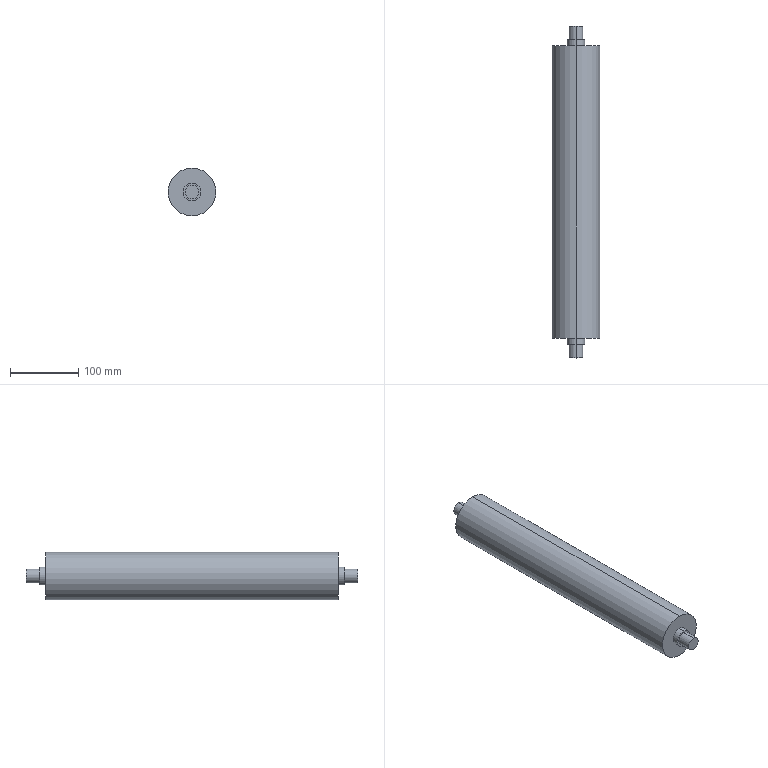Part | STEP file | 1.6米滚轮1 | 1 solid | 16 faces | box 70 x 486 x 70 mm | volume 1669260 mm3 | cylinder 10 | plane 6 | commonest cylinder face diameters 20 x4 26 x4 70 x2
STEP:
#1=CARTESIAN_POINT('',(0.,-29.,10.));
#2=VERTEX_POINT('',#1);
#3=CARTESIAN_POINT('',(0.,-29.,-10.));
#4=VERTEX_POINT('',#3);
#5=CARTESIAN_POINT('',(0.,-29.,0.));
#6=DIRECTION('',(0.,1.,0.));
#7=DIRECTION('',(0.,0.,1.));
#8=AXIS2_PLACEMENT_3D('',#5,#6,#7);
#9=CIRCLE('',#8,10.);
#10=EDGE_CURVE('',#2,#4,#9,.T.);
#11=ORIENTED_EDGE('',*,*,#10,.T.);
#12=CARTESIAN_POINT('',(0.,-9.,-10.));
#13=VERTEX_POINT('',#12);
#14=CARTESIAN_POINT('',(0.,-29.,-10.));
#15=DIRECTION('',(0.,1.,0.));
#16=VECTOR('',#15,1000.);
#17=LINE('',#14,#16);
#18=EDGE_CURVE('',#4,#13,#17,.T.);
#19=ORIENTED_EDGE('',*,*,#18,.T.);
#20=CARTESIAN_POINT('',(0.,-9.,10.));
#21=VERTEX_POINT('',#20);
#22=CARTESIAN_POINT('',(0.,-9.,0.));
#23=DIRECTION('',(0.,-1.,0.));
#24=DIRECTION('',(0.,0.,-1.));
#25=AXIS2_PLACEMENT_3D('',#22,#23,#24);
#26=CIRCLE('',#25,10.);
#27=EDGE_CURVE('',#13,#21,#26,.T.);
#28=ORIENTED_EDGE('',*,*,#27,.T.);
#29=CARTESIAN_POINT('',(0.,-29.,10.));
#30=DIRECTION('',(0.,1.,0.));
#31=VECTOR('',#30,1000.);
#32=LINE('',#29,#31);
#33=EDGE_CURVE('',#2,#21,#32,.T.);
#34=ORIENTED_EDGE('',*,*,#33,.F.);
#35=EDGE_LOOP('',(#11,#19,#28,#34));
#36=FACE_OUTER_BOUND('',#35,.T.);
#37=CARTESIAN_POINT('',(0.,-29.,0.));
#38=DIRECTION('',(0.,1.,0.));
#39=DIRECTION('',(0.,0.,1.));
#40=AXIS2_PLACEMENT_3D('',#37,#38,#39);
#41=CYLINDRICAL_SURFACE('',#40,10.);
#42=ADVANCED_FACE('',(#36),#41,.T.);
#43=CARTESIAN_POINT('',(0.,-9.,13.));
#44=VERTEX_POINT('',#43);
#45=CARTESIAN_POINT('',(0.,-9.,-13.));
#46=VERTEX_POINT('',#45);
#47=CARTESIAN_POINT('',(0.,-9.,0.));
#48=DIRECTION('',(0.,1.,0.));
#49=DIRECTION('',(0.,0.,1.));
#50=AXIS2_PLACEMENT_3D('',#47,#48,#49);
#51=CIRCLE('',#50,13.);
#52=EDGE_CURVE('',#44,#46,#51,.T.);
#53=ORIENTED_EDGE('',*,*,#52,.T.);
#54=CARTESIAN_POINT('',(0.,0.,-13.));
#55=VERTEX_POINT('',#54);
#56=CARTESIAN_POINT('',(0.,-9.,-13.));
#57=DIRECTION('',(0.,1.,0.));
#58=VECTOR('',#57,1000.);
#59=LINE('',#56,#58);
#60=EDGE_CURVE('',#46,#55,#59,.T.);
#61=ORIENTED_EDGE('',*,*,#60,.T.);
#62=CARTESIAN_POINT('',(0.,0.,13.));
#63=VERTEX_POINT('',#62);
#64=CARTESIAN_POINT('',(0.,0.,0.));
#65=DIRECTION('',(0.,1.,0.));
#66=DIRECTION('',(0.,0.,1.));
#67=AXIS2_PLACEMENT_3D('',#64,#65,#66);
#68=CIRCLE('',#67,13.);
#69=EDGE_CURVE('',#63,#55,#68,.T.);
#70=ORIENTED_EDGE('',*,*,#69,.F.);
#71=CARTESIAN_POINT('',(0.,-9.,13.));
#72=DIRECTION('',(0.,1.,0.));
#73=VECTOR('',#72,1000.);
#74=LINE('',#71,#73);
#75=EDGE_CURVE('',#44,#63,#74,.T.);
#76=ORIENTED_EDGE('',*,*,#75,.F.);
#77=EDGE_LOOP('',(#53,#61,#70,#76));
#78=FACE_OUTER_BOUND('',#77,.T.);
#79=CARTESIAN_POINT('',(0.,-9.,0.));
#80=DIRECTION('',(0.,1.,0.));
#81=DIRECTION('',(0.,0.,1.));
#82=AXIS2_PLACEMENT_3D('',#79,#80,#81);
#83=CYLINDRICAL_SURFACE('',#82,13.);
#84=ADVANCED_FACE('',(#78),#83,.T.);
#85=CARTESIAN_POINT('',(0.,457.,10.));
#86=VERTEX_POINT('',#85);
#87=CARTESIAN_POINT('',(0.,457.,-10.));
#88=VERTEX_POINT('',#87);
#89=CARTESIAN_POINT('',(0.,457.,0.));
#90=DIRECTION('',(0.,1.,0.));
#91=DIRECTION('',(0.,0.,1.));
#92=AXIS2_PLACEMENT_3D('',#89,#90,#91);
#93=CIRCLE('',#92,10.);
#94=EDGE_CURVE('',#86,#88,#93,.T.);
#95=ORIENTED_EDGE('',*,*,#94,.F.);
#96=CARTESIAN_POINT('',(0.,437.,10.));
#97=VERTEX_POINT('',#96);
#98=CARTESIAN_POINT('',(0.,457.,10.));
#99=DIRECTION('',(0.,-1.,0.));
#100=VECTOR('',#99,1000.);
#101=LINE('',#98,#100);
#102=EDGE_CURVE('',#86,#97,#101,.T.);
#103=ORIENTED_EDGE('',*,*,#102,.T.);
#104=CARTESIAN_POINT('',(0.,437.,-10.));
#105=VERTEX_POINT('',#104);
#106=CARTESIAN_POINT('',(0.,437.,0.));
#107=DIRECTION('',(0.,1.,0.));
#108=DIRECTION('',(0.,0.,1.));
#109=AXIS2_PLACEMENT_3D('',#106,#107,#108);
#110=CIRCLE('',#109,10.);
#111=EDGE_CURVE('',#97,#105,#110,.T.);
#112=ORIENTED_EDGE('',*,*,#111,.T.);
#113=CARTESIAN_POINT('',(0.,457.,-10.));
#114=DIRECTION('',(0.,-1.,0.));
#115=VECTOR('',#114,1000.);
#116=LINE('',#113,#115);
#117=EDGE_CURVE('',#88,#105,#116,.T.);
#118=ORIENTED_EDGE('',*,*,#117,.F.);
#119=EDGE_LOOP('',(#95,#103,#112,#118));
#120=FACE_OUTER_BOUND('',#119,.T.);
#121=CARTESIAN_POINT('',(0.,457.,0.));
#122=DIRECTION('',(0.,-1.,0.));
#123=DIRECTION('',(0.,0.,-1.));
#124=AXIS2_PLACEMENT_3D('',#121,#122,#123);
#125=CYLINDRICAL_SURFACE('',#124,10.);
#126=ADVANCED_FACE('',(#120),#125,.T.);
#127=CARTESIAN_POINT('',(0.,437.,13.));
#128=VERTEX_POINT('',#127);
#129=CARTESIAN_POINT('',(0.,437.,-13.));
#130=VERTEX_POINT('',#129);
#131=CARTESIAN_POINT('',(0.,437.,0.));
#132=DIRECTION('',(0.,1.,0.));
#133=DIRECTION('',(0.,0.,1.));
#134=AXIS2_PLACEMENT_3D('',#131,#132,#133);
#135=CIRCLE('',#134,13.);
#136=EDGE_CURVE('',#128,#130,#135,.T.);
#137=ORIENTED_EDGE('',*,*,#136,.F.);
#138=CARTESIAN_POINT('',(0.,428.,13.));
#139=VERTEX_POINT('',#138);
#140=CARTESIAN_POINT('',(0.,437.,13.));
#141=DIRECTION('',(0.,-1.,0.));
#142=VECTOR('',#141,1000.);
#143=LINE('',#140,#142);
#144=EDGE_CURVE('',#128,#139,#143,.T.);
#145=ORIENTED_EDGE('',*,*,#144,.T.);
#146=CARTESIAN_POINT('',(0.,428.,-13.));
#147=VERTEX_POINT('',#146);
#148=CARTESIAN_POINT('',(0.,428.,0.));
#149=DIRECTION('',(0.,1.,0.));
#150=DIRECTION('',(0.,0.,1.));
#151=AXIS2_PLACEMENT_3D('',#148,#149,#150);
#152=CIRCLE('',#151,13.);
#153=EDGE_CURVE('',#139,#147,#152,.T.);
#154=ORIENTED_EDGE('',*,*,#153,.T.);
#155=CARTESIAN_POINT('',(0.,437.,-13.));
#156=DIRECTION('',(0.,-1.,0.));
#157=VECTOR('',#156,1000.);
#158=LINE('',#155,#157);
#159=EDGE_CURVE('',#130,#147,#158,.T.);
#160=ORIENTED_EDGE('',*,*,#159,.F.);
#161=EDGE_LOOP('',(#137,#145,#154,#160));
#162=FACE_OUTER_BOUND('',#161,.T.);
#163=CARTESIAN_POINT('',(0.,437.,0.));
#164=DIRECTION('',(0.,-1.,0.));
#165=DIRECTION('',(0.,0.,-1.));
#166=AXIS2_PLACEMENT_3D('',#163,#164,#165);
#167=CYLINDRICAL_SURFACE('',#166,13.);
#168=ADVANCED_FACE('',(#162),#167,.T.);
#169=CARTESIAN_POINT('',(0.,428.,35.));
#170=VERTEX_POINT('',#169);
#171=CARTESIAN_POINT('',(0.,428.,-35.));
#172=VERTEX_POINT('',#171);
#173=CARTESIAN_POINT('',(0.,428.,0.));
#174=DIRECTION('',(0.,1.,0.));
#175=DIRECTION('',(0.,0.,1.));
#176=AXIS2_PLACEMENT_3D('',#173,#174,#175);
#177=CIRCLE('',#176,35.);
#178=EDGE_CURVE('',#170,#172,#177,.T.);
#179=ORIENTED_EDGE('',*,*,#178,.F.);
#180=CARTESIAN_POINT('',(0.,0.,35.));
#181=VERTEX_POINT('',#180);
#182=CARTESIAN_POINT('',(0.,428.,35.));
#183=DIRECTION('',(0.,-1.,0.));
#184=VECTOR('',#183,1000.);
#185=LINE('',#182,#184);
#186=EDGE_CURVE('',#170,#181,#185,.T.);
#187=ORIENTED_EDGE('',*,*,#186,.T.);
#188=CARTESIAN_POINT('',(0.,0.,-35.));
#189=VERTEX_POINT('',#188);
#190=CARTESIAN_POINT('',(0.,0.,0.));
#191=DIRECTION('',(0.,1.,0.));
#192=DIRECTION('',(0.,0.,1.));
#193=AXIS2_PLACEMENT_3D('',#190,#191,#192);
#194=CIRCLE('',#193,35.);
#195=EDGE_CURVE('',#181,#189,#194,.T.);
#196=ORIENTED_EDGE('',*,*,#195,.T.);
#197=CARTESIAN_POINT('',(0.,428.,-35.));
#198=DIRECTION('',(0.,-1.,0.));
#199=VECTOR('',#198,1000.);
#200=LINE('',#197,#199);
#201=EDGE_CURVE('',#172,#189,#200,.T.);
#202=ORIENTED_EDGE('',*,*,#201,.F.);
#203=EDGE_LOOP('',(#179,#187,#196,#202));
#204=FACE_OUTER_BOUND('',#203,.T.);
#205=CARTESIAN_POINT('',(0.,428.,0.));
#206=DIRECTION('',(0.,-1.,0.));
#207=DIRECTION('',(0.,0.,-1.));
#208=AXIS2_PLACEMENT_3D('',#205,#206,#207);
#209=CYLINDRICAL_SURFACE('',#208,35.);
#210=ADVANCED_FACE('',(#204),#209,.T.);
#211=ORIENTED_EDGE('',*,*,#186,.F.);
#212=CARTESIAN_POINT('',(0.,428.,0.));
#213=DIRECTION('',(0.,1.,0.));
#214=DIRECTION('',(0.,0.,1.));
#215=AXIS2_PLACEMENT_3D('',#212,#213,#214);
#216=CIRCLE('',#215,35.);
#217=EDGE_CURVE('',#172,#170,#216,.T.);
#218=ORIENTED_EDGE('',*,*,#217,.F.);
#219=ORIENTED_EDGE('',*,*,#201,.T.);
#220=CARTESIAN_POINT('',(0.,0.,0.));
#221=DIRECTION('',(0.,1.,0.));
#222=DIRECTION('',(0.,0.,1.));
#223=AXIS2_PLACEMENT_3D('',#220,#221,#222);
#224=CIRCLE('',#223,35.);
#225=EDGE_CURVE('',#189,#181,#224,.T.);
#226=ORIENTED_EDGE('',*,*,#225,.T.);
#227=EDGE_LOOP('',(#211,#218,#219,#226));
#228=FACE_OUTER_BOUND('',#227,.T.);
#229=CARTESIAN_POINT('',(0.,428.,0.));
#230=DIRECTION('',(0.,-1.,0.));
#231=DIRECTION('',(0.,0.,-1.));
#232=AXIS2_PLACEMENT_3D('',#229,#230,#231);
#233=CYLINDRICAL_SURFACE('',#232,35.);
#234=ADVANCED_FACE('',(#228),#233,.T.);
#235=CARTESIAN_POINT('',(0.,428.,0.));
#236=DIRECTION('',(0.,1.,0.));
#237=DIRECTION('',(0.,0.,1.));
#238=AXIS2_PLACEMENT_3D('',#235,#236,#237);
#239=CIRCLE('',#238,13.);
#240=EDGE_CURVE('',#147,#139,#239,.T.);
#241=ORIENTED_EDGE('',*,*,#240,.F.);
#242=ORIENTED_EDGE('',*,*,#153,.F.);
#243=EDGE_LOOP('',(#241,#242));
#244=FACE_BOUND('',#243,.T.);
#245=ORIENTED_EDGE('',*,*,#217,.T.);
#246=ORIENTED_EDGE('',*,*,#178,.T.);
#247=EDGE_LOOP('',(#245,#246));
#248=FACE_OUTER_BOUND('',#247,.T.);
#249=CARTESIAN_POINT('',(0.,428.,0.));
#250=DIRECTION('',(0.,1.,0.));
#251=DIRECTION('',(0.,0.,1.));
#252=AXIS2_PLACEMENT_3D('',#249,#250,#251);
#253=PLANE('',#252);
#254=ADVANCED_FACE('',(#244,#248),#253,.T.);
#255=ORIENTED_EDGE('',*,*,#69,.T.);
#256=CARTESIAN_POINT('',(0.,0.,0.));
#257=DIRECTION('',(0.,1.,0.));
#258=DIRECTION('',(0.,0.,1.));
#259=AXIS2_PLACEMENT_3D('',#256,#257,#258);
#260=CIRCLE('',#259,13.);
#261=EDGE_CURVE('',#55,#63,#260,.T.);
#262=ORIENTED_EDGE('',*,*,#261,.T.);
#263=EDGE_LOOP('',(#255,#262));
#264=FACE_BOUND('',#263,.T.);
#265=ORIENTED_EDGE('',*,*,#225,.F.);
#266=ORIENTED_EDGE('',*,*,#195,.F.);
#267=EDGE_LOOP('',(#265,#266));
#268=FACE_OUTER_BOUND('',#267,.T.);
#269=CARTESIAN_POINT('',(0.,0.,0.));
#270=DIRECTION('',(0.,1.,0.));
#271=DIRECTION('',(0.,0.,1.));
#272=AXIS2_PLACEMENT_3D('',#269,#270,#271);
#273=PLANE('',#272);
#274=ADVANCED_FACE('',(#264,#268),#273,.F.);
#275=ORIENTED_EDGE('',*,*,#144,.F.);
#276=CARTESIAN_POINT('',(0.,437.,0.));
#277=DIRECTION('',(0.,1.,0.));
#278=DIRECTION('',(0.,0.,1.));
#279=AXIS2_PLACEMENT_3D('',#276,#277,#278);
#280=CIRCLE('',#279,13.);
#281=EDGE_CURVE('',#130,#128,#280,.T.);
#282=ORIENTED_EDGE('',*,*,#281,.F.);
#283=ORIENTED_EDGE('',*,*,#159,.T.);
#284=ORIENTED_EDGE('',*,*,#240,.T.);
#285=EDGE_LOOP('',(#275,#282,#283,#284));
#286=FACE_OUTER_BOUND('',#285,.T.);
#287=CARTESIAN_POINT('',(0.,437.,0.));
#288=DIRECTION('',(0.,-1.,0.));
#289=DIRECTION('',(0.,0.,-1.));
#290=AXIS2_PLACEMENT_3D('',#287,#288,#289);
#291=CYLINDRICAL_SURFACE('',#290,13.);
#292=ADVANCED_FACE('',(#286),#291,.T.);
#293=CARTESIAN_POINT('',(0.,437.,0.));
#294=DIRECTION('',(0.,1.,0.));
#295=DIRECTION('',(0.,0.,1.));
#296=AXIS2_PLACEMENT_3D('',#293,#294,#295);
#297=CIRCLE('',#296,10.);
#298=EDGE_CURVE('',#105,#97,#297,.T.);
#299=ORIENTED_EDGE('',*,*,#298,.F.);
#300=ORIENTED_EDGE('',*,*,#111,.F.);
#301=EDGE_LOOP('',(#299,#300));
#302=FACE_BOUND('',#301,.T.);
#303=ORIENTED_EDGE('',*,*,#281,.T.);
#304=ORIENTED_EDGE('',*,*,#136,.T.);
#305=EDGE_LOOP('',(#303,#304));
#306=FACE_OUTER_BOUND('',#305,.T.);
#307=CARTESIAN_POINT('',(0.,437.,0.));
#308=DIRECTION('',(0.,1.,0.));
#309=DIRECTION('',(0.,0.,1.));
#310=AXIS2_PLACEMENT_3D('',#307,#308,#309);
#311=PLANE('',#310);
#312=ADVANCED_FACE('',(#302,#306),#311,.T.);
#313=ORIENTED_EDGE('',*,*,#102,.F.);
#314=CARTESIAN_POINT('',(0.,457.,0.));
#315=DIRECTION('',(0.,1.,0.));
#316=DIRECTION('',(0.,0.,1.));
#317=AXIS2_PLACEMENT_3D('',#314,#315,#316);
#318=CIRCLE('',#317,10.);
#319=EDGE_CURVE('',#88,#86,#318,.T.);
#320=ORIENTED_EDGE('',*,*,#319,.F.);
#321=ORIENTED_EDGE('',*,*,#117,.T.);
#322=ORIENTED_EDGE('',*,*,#298,.T.);
#323=EDGE_LOOP('',(#313,#320,#321,#322));
#324=FACE_OUTER_BOUND('',#323,.T.);
#325=CARTESIAN_POINT('',(0.,457.,0.));
#326=DIRECTION('',(0.,-1.,0.));
#327=DIRECTION('',(0.,0.,-1.));
#328=AXIS2_PLACEMENT_3D('',#325,#326,#327);
#329=CYLINDRICAL_SURFACE('',#328,10.);
#330=ADVANCED_FACE('',(#324),#329,.T.);
#331=ORIENTED_EDGE('',*,*,#319,.T.);
#332=ORIENTED_EDGE('',*,*,#94,.T.);
#333=EDGE_LOOP('',(#331,#332));
#334=FACE_OUTER_BOUND('',#333,.T.);
#335=CARTESIAN_POINT('',(0.,457.,0.));
#336=DIRECTION('',(0.,1.,0.));
#337=DIRECTION('',(0.,0.,1.));
#338=AXIS2_PLACEMENT_3D('',#335,#336,#337);
#339=PLANE('',#338);
#340=ADVANCED_FACE('',(#334),#339,.T.);
#341=ORIENTED_EDGE('',*,*,#60,.F.);
#342=CARTESIAN_POINT('',(0.,-9.,0.));
#343=DIRECTION('',(0.,1.,0.));
#344=DIRECTION('',(0.,0.,1.));
#345=AXIS2_PLACEMENT_3D('',#342,#343,#344);
#346=CIRCLE('',#345,13.);
#347=EDGE_CURVE('',#46,#44,#346,.T.);
#348=ORIENTED_EDGE('',*,*,#347,.T.);
#349=ORIENTED_EDGE('',*,*,#75,.T.);
#350=ORIENTED_EDGE('',*,*,#261,.F.);
#351=EDGE_LOOP('',(#341,#348,#349,#350));
#352=FACE_OUTER_BOUND('',#351,.T.);
#353=CARTESIAN_POINT('',(0.,-9.,0.));
#354=DIRECTION('',(0.,1.,0.));
#355=DIRECTION('',(0.,0.,1.));
#356=AXIS2_PLACEMENT_3D('',#353,#354,#355);
#357=CYLINDRICAL_SURFACE('',#356,13.);
#358=ADVANCED_FACE('',(#352),#357,.T.);
#359=CARTESIAN_POINT('',(0.,-9.,0.));
#360=DIRECTION('',(0.,-1.,0.));
#361=DIRECTION('',(0.,0.,-1.));
#362=AXIS2_PLACEMENT_3D('',#359,#360,#361);
#363=CIRCLE('',#362,10.);
#364=EDGE_CURVE('',#21,#13,#363,.T.);
#365=ORIENTED_EDGE('',*,*,#364,.F.);
#366=ORIENTED_EDGE('',*,*,#27,.F.);
#367=EDGE_LOOP('',(#365,#366));
#368=FACE_BOUND('',#367,.T.);
#369=ORIENTED_EDGE('',*,*,#52,.F.);
#370=ORIENTED_EDGE('',*,*,#347,.F.);
#371=EDGE_LOOP('',(#369,#370));
#372=FACE_OUTER_BOUND('',#371,.T.);
#373=CARTESIAN_POINT('',(0.,-9.,0.));
#374=DIRECTION('',(0.,-1.,0.));
#375=DIRECTION('',(0.,0.,1.));
#376=AXIS2_PLACEMENT_3D('',#373,#374,#375);
#377=PLANE('',#376);
#378=ADVANCED_FACE('',(#368,#372),#377,.T.);
#379=ORIENTED_EDGE('',*,*,#18,.F.);
#380=CARTESIAN_POINT('',(0.,-29.,0.));
#381=DIRECTION('',(0.,1.,0.));
#382=DIRECTION('',(0.,0.,1.));
#383=AXIS2_PLACEMENT_3D('',#380,#381,#382);
#384=CIRCLE('',#383,10.);
#385=EDGE_CURVE('',#4,#2,#384,.T.);
#386=ORIENTED_EDGE('',*,*,#385,.T.);
#387=ORIENTED_EDGE('',*,*,#33,.T.);
#388=ORIENTED_EDGE('',*,*,#364,.T.);
#389=EDGE_LOOP('',(#379,#386,#387,#388));
#390=FACE_OUTER_BOUND('',#389,.T.);
#391=CARTESIAN_POINT('',(0.,-29.,0.));
#392=DIRECTION('',(0.,1.,0.));
#393=DIRECTION('',(0.,0.,1.));
#394=AXIS2_PLACEMENT_3D('',#391,#392,#393);
#395=CYLINDRICAL_SURFACE('',#394,10.);
#396=ADVANCED_FACE('',(#390),#395,.T.);
#397=ORIENTED_EDGE('',*,*,#10,.F.);
#398=ORIENTED_EDGE('',*,*,#385,.F.);
#399=EDGE_LOOP('',(#397,#398));
#400=FACE_OUTER_BOUND('',#399,.T.);
#401=CARTESIAN_POINT('',(0.,-29.,0.));
#402=DIRECTION('',(0.,-1.,0.));
#403=DIRECTION('',(0.,0.,1.));
#404=AXIS2_PLACEMENT_3D('',#401,#402,#403);
#405=PLANE('',#404);
#406=ADVANCED_FACE('',(#400),#405,.T.);
#407=CLOSED_SHELL('',(#42,#84,#126,#168,#210,#234,#254,#274,#292,#312,#330,#340,#358,#378,#396,#406));
#408=MANIFOLD_SOLID_BREP('',#407);
#409=CARTESIAN_POINT('',(0.,0.,0.));
#410=DIRECTION('',(0.,0.,1.));
#411=DIRECTION('',(1.,0.,0.));
#412=AXIS2_PLACEMENT_3D('',#409,#410,#411);
#413=(LENGTH_UNIT()NAMED_UNIT(*)SI_UNIT(.MILLI.,.METRE.));
#414=UNCERTAINTY_MEASURE_WITH_UNIT(LENGTH_MEASURE(0.00001),#413,'','');
#415=(NAMED_UNIT(*)PLANE_ANGLE_UNIT()SI_UNIT($,.RADIAN.));
#416=(NAMED_UNIT(*)SI_UNIT($,.STERADIAN.)SOLID_ANGLE_UNIT());
#417=(GEOMETRIC_REPRESENTATION_CONTEXT(3)GLOBAL_UNCERTAINTY_ASSIGNED_CONTEXT((#414))GLOBAL_UNIT_ASSIGNED_CONTEXT((#413,#415,#416))REPRESENTATION_CONTEXT('',''));
#418=ADVANCED_BREP_SHAPE_REPRESENTATION('',(#408,#412),#417);